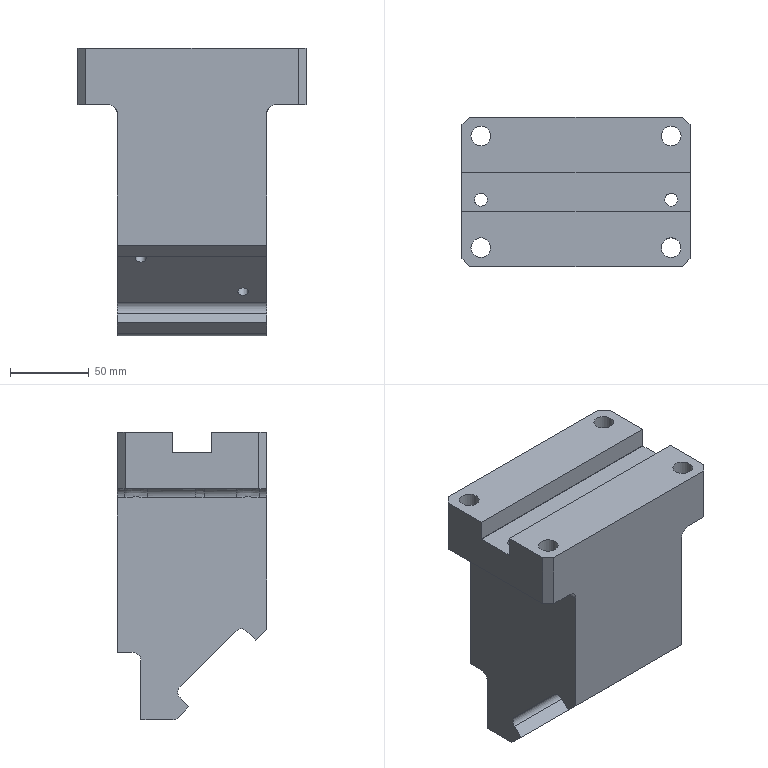Part | STEP file | 1_id166_x_t | 1 solid | 71 faces | box 145 x 95 x 182.773 mm | volume 1439851 mm3 | plane 31 | cylinder 30 | spline 6 | cone 4 | commonest cylinder face diameters 12 x8 6.75 x4 10 x4 12.5 x4 20 x4 0.4 x2